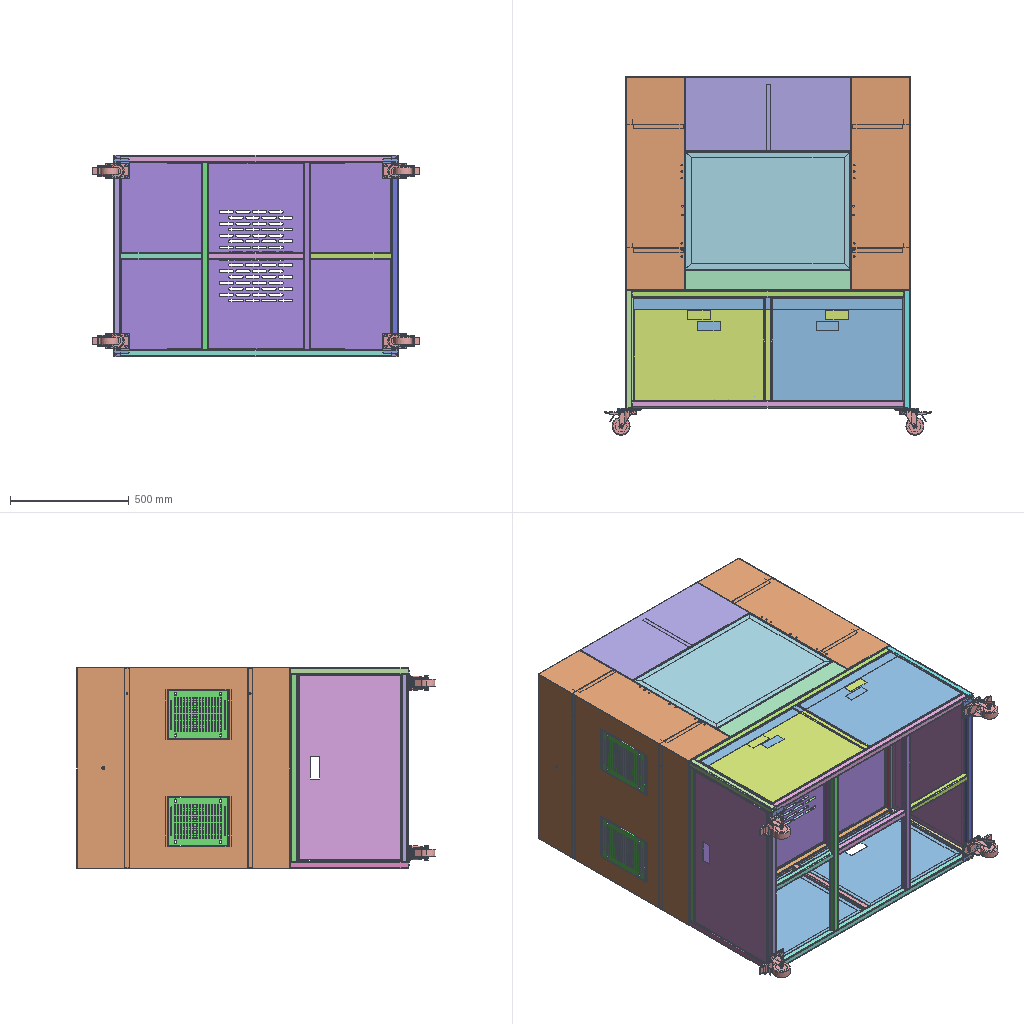Assembly | SolidWorks | 33 different items | 82 placed | box 1381 x 1511 x 850 mm
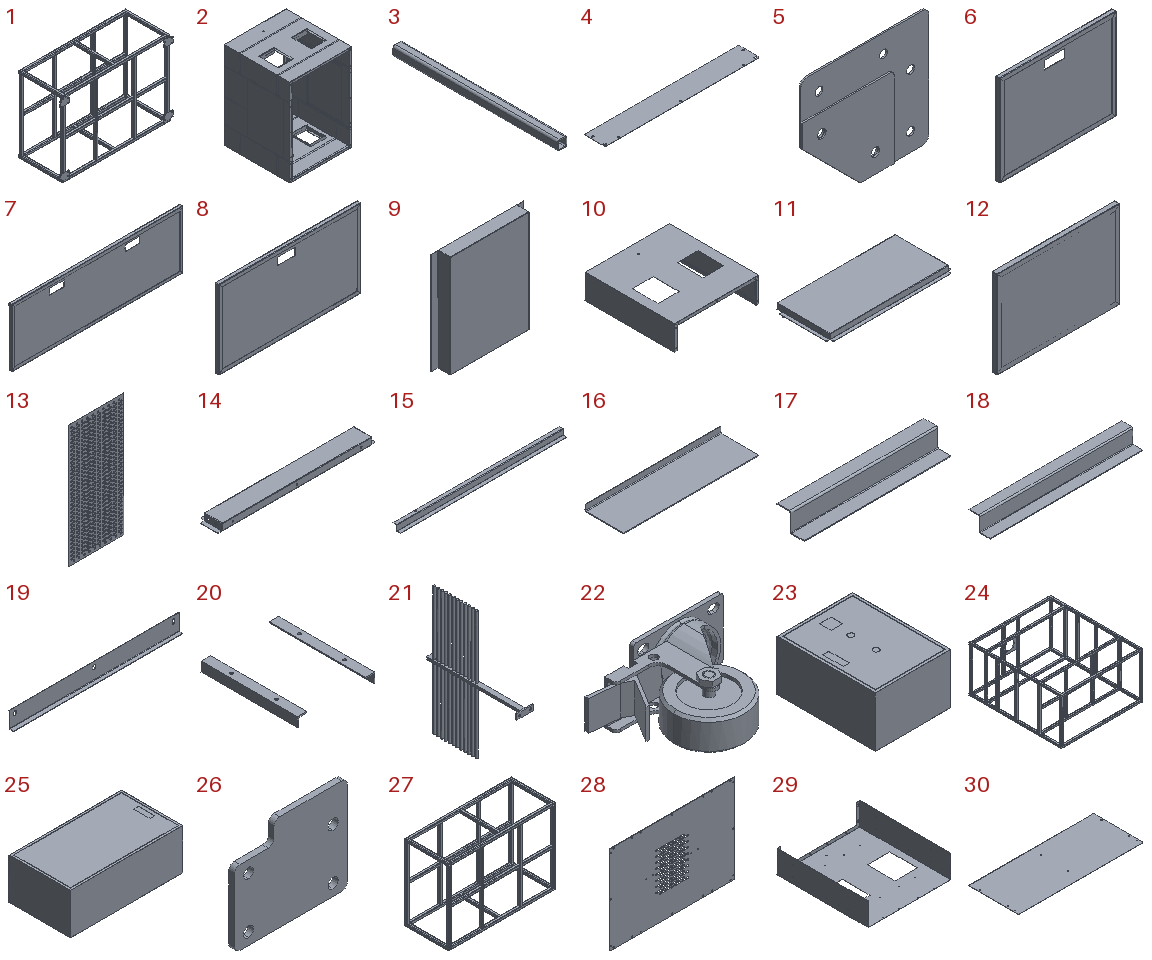Parts list (item | name | quantity | parent item | size | volume | features):
1 | (subassembly) | x1 | - | 1270 x 501 x 850 mm | 4402575 mm3 | features ReferencePattern 2, AEMSimFeature 1, LocalLPattern 1
2 | (subassembly) | x1 | - | 850 x 900 x 1200 mm | 10155913 mm3 | features ReferencePattern 29, MirrorCompFeat 4, LocalLPattern 2, AEMSimFeature 1
3 | - | x1 | - | 30 x 520 x 30 mm | 164668 mm3 | features HoleWzd 1, ICE 1, WeldMemberFeat 1, WeldmentFeature 1
4 | - | x2 | in 2 | 745 x 100 x 1.2 mm | 88883 mm3 | features EdgeFlange 2, Fillet 1, FlatPattern 1, HoleWzd 1, ICE 1, SMBaseFlange 1, SheetMetal 1
5 | - | x1 | - | 99 x 2.4 x 90.5 mm | 13339 mm3 | features ICE 9, EdgeFlange 2, Fillet 2, HoleWzd 2, FlatPattern 1, SMBaseFlange 1, SheetMetal 1, WeldmentFeature 1
6 | - | x4 | - | 552 x 20 x 432 mm | 364714 mm3 | features EdgeFlange 2, FlatPattern 1, ICE 1, SMBaseFlange 1, SheetMetal 1
7 | - | x1 | - | 1135 x 20 x 386 mm | 646370 mm3 | features EdgeFlange 2, FlatPattern 1, ICE 1, SMBaseFlange 1, SheetMetal 1
8 | - | x2 | - | 782 x 20 x 432 mm | 503943 mm3 | features EdgeFlange 2, FlatPattern 1, ICE 1, SMBaseFlange 1, SheetMetal 1
9 | - | x1 | in 1 | 457 x 62.2 x 504.4 mm | 401697 mm3 | features EdgeFlange 2, FlatPattern 1, SMBaseFlange 1, SheetMetal 1
10 | - | x2 | in 2 | 850 x 900 x 250 mm | 1614034 mm3 | features EdgeFlange 8, ICE 5, HoleWzd 4, Fillet 1, FlatPattern 1, LPattern 1, SMBaseFlange 1, SheetMetal 1
11 | - | x2 | in 2 | 737.6 x 333.8 x 60.8 mm | 412436 mm3 | features EdgeFlange 5, ICE 2, Fillet 1, FlatPattern 1, HoleWzd 1, SMBaseFlange 1, SheetMetal 1
12 | - | x2 | in 2 | 696 x 29.2 x 496 mm | 963992 mm3 | features EdgeFlange 2, FlatPattern 1, HoleWzd 1, ICE 1, SMBaseFlange 1, SheetMetal 1
13 | - | x1 | - | 497 x 1.2 x 1097 mm | 505811 mm3 | features LPattern 2, FlatPattern 1, ICE 1, SMBaseFlange 1, SheetMetal 1
14 | - | x2 | in 2 | 737.6 x 103.8 x 32 mm | 156480 mm3 | features EdgeFlange 6, Fillet 1, FlatPattern 1, HoleWzd 1, ICE 1, SMBaseFlange 1, SheetMetal 1
15 | - | x4 | in 2 | 843 x 38.8 x 28.5 mm | 65431 mm3 | features EdgeFlange 2, FlatPattern 1, HoleWzd 1, SMBaseFlange 1, SheetMetal 1
16 | - | x8 | in 2 | 209 x 60 x 10 mm | 17083 mm3 | features EdgeFlange 1, FlatPattern 1, HoleWzd 1, SMBaseFlange 1, SheetMetal 1
17 | - | x8 | in 2 | 210 x 38.8 x 28 mm | 16185 mm3 | features EdgeFlange 2, FlatPattern 1, HoleWzd 1, SMBaseFlange 1, SheetMetal 1
18 | - | x2 | in 2 | 281 x 38.8 x 28 mm | 21657 mm3 | features EdgeFlange 2, FlatPattern 1, HoleWzd 1, SMBaseFlange 1, SheetMetal 1
19 | - | x4 | in 2 | 460 x 12 x 45 mm | 30158 mm3 | features EdgeFlange 2, Fillet 1, FlatPattern 1, ICE 1, LPattern 1, SMBaseFlange 1, SheetMetal 1
20 | - | x1 | in 2 | 205 x 255 x 25 mm | 72570 mm3 | features HoleWzd 1, WeldMemberFeat 1, WeldmentFeature 1
21 | - | x2 | - | 90 x 526 x 700 mm | 1128275 mm3 | features ICE 4, Extrusion 1, HoleWzd 1, LPattern 1
22 | - | x4 | in 1 | 152.5 x 108 x 64 mm | 200603 mm3 | features BaseBody 1
23 | - | x1 | - | 300 x 390 x 201 mm | 697946 mm3 | features ICE 2, Extrusion 1, Shell 1
24 | - | x1 | in 1 | 1200 x 1370 x 680 mm | 7177358 mm3 | features 3DProfileFeature 1, HoleWzd 1, ICE 1, WeldMemberFeat 1, WeldmentFeature 1
25 | - | x1 | - | 550 x 300 x 201 mm | 911866 mm3 | features ICE 3, Extrusion 1, Shell 1
26 | - | x4 | in 1 | 100 x 5 x 85 mm | 37795 mm3 | features Fillet 2, Extrusion 1, HoleWzd 1, ICE 1
27 | - | x1 | in 1 | 1200 x 495 x 850 mm | 4251393 mm3 | features WeldCornerFeat 2, 3DProfileFeature 1, WeldMemberFeat 1, WeldmentFeature 1
28 | - | x1 | - | 1196 x 1.2 x 846 mm | 1157126 mm3 | features LPattern 4, HoleWzd 3, EdgeFlange 1, Fillet 1, FlatPattern 1, ICE 1, SMBaseFlange 1, SheetMetal 1
29 | - | x2 | in 2 | 787 x 866 x 220 mm | 1173690 mm3 | features ICE 6, HoleWzd 5, EdgeFlange 4, LPattern 2, Fillet 1, FlatPattern 1, SMBaseFlange 1, SheetMetal 1
30 | - | x2 | in 2 | 745 x 300 x 30 mm | 291345 mm3 | features EdgeFlange 2, HoleWzd 2, Fillet 1, FlatPattern 1, SMBaseFlange 1, SheetMetal 1
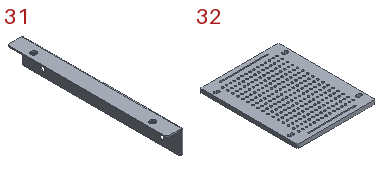31 | - | x8 | in 2 | 26 x 255 x 40 mm | 31191 mm3 | features ICE 2, EdgeFlange 1, Fillet 1, FlatPattern 1, SMBaseFlange 1, SheetMetal 1
32 | - | x4 | - | 200 x 250 x 10 mm | 441110 mm3 | features ICE 3, LPattern 3, Chamfer 1, Extrusion 1
33 | CBAhxj04-2 | x1 | - | - | - | -
Mates (type | each side: item.copy, entity, surface, feature):
In the top assembly
Coincident | 24.1 face plane Square Tube 30 X 30 X 2.6(1) | assembly face | 12 times
Coincident | 24.1 face plane Boss-Extrude1 | assembly face
Concentric | 24.1 face cylinder Boss-Extrude1 | assembly face
Concentric | 24.1 face cylinder M10 Tapped Hole1 | assembly face
DistanceDim | 27.1 face plane Square Tube 30 X 30 X 2.6 - missing(1) | 10.1 face plane Edge-Flange2
Coincident | 27.1 face plane Square Tube 30 X 30 X 2.6 - missing(1) | 10.1 face plane Base-Flange1
Coincident | 27.1 face plane Square Tube 30 X 30 X 2.6 - missing(1) | 10.1 face plane Edge-Flange1
Coincident | 27.1 face plane Square Tube 30 X 30 X 2.6 - missing(1) | 21.1 face plane Boss-Extrude3
Coincident | 27.1 face plane Square Tube 30 X 30 X 2.6 - missing(1) | 21.1 face plane Boss-Extrude1
Coincident | 21.1 face plane Boss-Extrude3 | 21.2 face plane Boss-Extrude3
Coincident | 27.1 face plane Square Tube 30 X 30 X 2.6 - missing(1) | 21.2 face plane Boss-Extrude1
Coincident | 21.1 face plane Boss-Extrude1 | 21.2 face plane Boss-Extrude1
DistanceDim | 27.1 face plane Square Tube 30 X 30 X 2.6 - missing(1) | 28.1 face plane Base-Flange1 | 2 times
Coincident | 28.1 face plane Base-Flange1 | assembly face
Coincident | 29.1 face plane Base-Flange1 | assembly face
Coincident | 28.1 face plane Base-Flange1 | 31.1 face
Coincident | 29.1 face plane Base-Flange1 | 31.1 face
Coincident | 29.2 face plane Base-Flange1 | 31.2 face
Coincident | 28.1 face plane Base-Flange1 | 31.2 face
Coincident | 31.1 face | 31.2 face
Width | 27.1 face plane Square Tube 30 X 30 X 2.6 - missing(1) | 27.1 face plane Square Tube 30 X 30 X 2.6 - missing(1) | 21.2 face plane Boss-Extrude1 | 21.2 face plane Boss-Extrude1
Coincident | 10.2 face plane Edge-Flange1 | 23.1 face
Coincident | 27.1 face plane Square Tube 30 X 30 X 2.6 - missing(1) | 23.1 face | 2 times
Coincident | 27.1 face plane Square Tube 30 X 30 X 2.6 - missing(1) | 6.1 face plane Edge-Flange1
DistanceDim | 6.1 face plane Edge-Flange1 | 27.1 face plane Square Tube 30 X 30 X 2.6 - missing(1)
Coincident | 27.1 face plane Square Tube 30 X 30 X 2.6 - missing(1) | 6.1 face plane Base-Flange1
Coincident | 27.1 face plane Square Tube 30 X 30 X 2.6 - missing(1) | 7.1 face plane Base-Flange1
Coincident | 27.1 face plane Square Tube 30 X 30 X 2.6 - missing(1) | 7.1 face plane Edge-Flange1
DistanceDim | 7.1 face plane Edge-Flange1 | 27.1 face plane Square Tube 30 X 30 X 2.6 - missing(1)
Coincident | 27.1 face plane Square Tube 30 X 30 X 2.6 - missing(1) | 8.1 face plane Edge-Flange1
Coincident | 27.1 face plane Square Tube 30 X 30 X 2.6 - missing(1) | 8.1 face plane Base-Flange1
DistanceDim | 8.1 face plane Edge-Flange1 | 27.1 face plane Square Tube 30 X 30 X 2.6 - missing(1)
Coincident | 27.1 face plane Square Tube 30 X 30 X 2.6 - missing(1) | 8.2 face plane Base-Flange1
Coincident | 27.1 face plane Square Tube 30 X 30 X 2.6 - missing(1) | 8.2 face plane Edge-Flange1
DistanceDim | 8.2 face plane Edge-Flange1 | 27.1 face plane Square Tube 30 X 30 X 2.6 - missing(1)
Coincident | 27.1 face plane Square Tube 30 X 30 X 2.6 - missing(1) | 28.1 face plane Base-Flange1
Coincident | 10.2 face plane Edge-Flange1 | 25.1 face
Coincident | 10.2 face plane Base-Flange1 | 25.1 face
Coincident | 10.2 face plane Edge-Flange2 | 5.1 face
Coincident | 10.2 face plane Edge-Flange2 | 5.2 face
DistanceDim | 10.1 face plane Edge-Flange2 | 5.3 face
Width | 3.1 face plane Square Tube 30 X 30 X 3.2(1) | 3.1 face plane Square Tube 30 X 30 X 3.2(1) | 21.2 face plane Boss-Extrude1 | 21.2 face plane Boss-Extrude1 | 2 times
Coincident | 21.2 face plane Boss-Extrude3 | 3.1 face plane Square Tube 30 X 30 X 3.2(1)
Coincident | 6.1 face plane Base-Flange1 | 6.2 face plane Base-Flange1
DistanceDim | 6.2 face plane Edge-Flange1 | 27.1 face plane Square Tube 30 X 30 X 2.6 - missing(1)
Coincident | 6.1 face plane Edge-Flange1 | 6.2 face plane Edge-Flange1
Coincident | 27.1 face plane Square Tube 30 X 30 X 2.6 - missing(1) | 6.3 face plane Base-Flange1
DistanceDim | 6.3 face plane Edge-Flange1 | 27.1 face plane Square Tube 30 X 30 X 2.6 - missing(1)
Coincident | 27.1 face plane Square Tube 30 X 30 X 2.6 - missing(1) | 6.3 face plane Edge-Flange1
Coincident | 6.3 face plane Base-Flange1 | 6.4 face plane Base-Flange1
DistanceDim | 6.4 face plane Edge-Flange1 | 27.1 face plane Square Tube 30 X 30 X 2.6 - missing(1)
Coincident | 6.3 face plane Edge-Flange1 | 6.4 face plane Edge-Flange1
Coincident | 31.3 face plane Base-Flange1 | 32.1 face plane Boss-Extrude1
Slot | 32.1 face cylinder Cut-Extrude3 | 31.3 face cylinder Cut-Extrude2 | 2 times
Parallel | 10.1 face plane Edge-Flange1 | 32.2 face plane Boss-Extrude1
Coincident | 31.4 face plane Base-Flange1 | 32.3 face plane Boss-Extrude1
Slot | 32.3 face cylinder Cut-Extrude3 | 31.4 face cylinder Cut-Extrude2
Slot | 32.3 face cylinder Cut-Extrude3 | 31.5 face cylinder Cut-Extrude2
In subassembly 2
Coincident | 10.3 face plane Edge-Flange1 | 10.4 face plane Edge-Flange1
DistanceDim | 10.3 face plane Base-Flange1 | 10.4 face plane Base-Flange1
Coincident | 10.3 face plane Edge-Flange2 | 10.4 face plane Edge-Flange2
Coincident | 10.3 face plane Edge-Flange1 | 11.1 face plane Base-Flange1
Coincident | 10.3 face plane Edge-Flange2 | 11.1 face plane Edge-Flange1 | 2 times
Coincident | 10.4 face plane Edge-Flange1 | 11.2 face plane Base-Flange1
Coincident | 10.4 face plane Edge-Flange2 | 11.2 face plane Edge-Flange1
Coincident | 10.3 face plane Edge-Flange9 | 29.3 face plane Base-Flange1
DistanceDim | 29.3 face plane Edge-Flange1 | 10.3 face plane Edge-Flange8
Coincident | 10.4 face plane Edge-Flange9 | 29.4 face plane Base-Flange1
Coincident | 29.3 face plane Edge-Flange1 | 29.4 face plane Edge-Flange1
Coincident | 11.2 face plane Edge-Flange5 | 30.1 face plane Base-Flange1
Coincident | 11.2 face plane Base-Flange1 | 12.1 face plane Base-Flange1
DistanceDim | 12.1 face plane Edge-Flange1 | 14.1 face plane Edge-Flange1
DistanceDim | 12.1 face plane Edge-Flange1 | 10.3 face plane Edge-Flange2
DistanceDim | 12.2 face plane Edge-Flange1 | 10.3 face plane Edge-Flange2
Coincident | 11.1 face plane Base-Flange1 | 12.2 face plane Boss-Extrude1
Coincident | 10.3 face plane Base-Flange1 | 15.1 face plane Edge-Flange2
DistanceDim | 10.3 face plane Edge-Flange2 | 15.1 face plane Edge-Flange1
DistanceDim | 15.1 face plane Edge-Flange1 | 10.3 face plane Edge-Flange1
Coincident | 10.3 face plane Edge-Flange2 | 29.3 face plane Edge-Flange1
Coincident | 10.4 face plane Edge-Flange2 | 29.4 face plane Edge-Flange1
DistanceDim | 10.3 face plane Cut-Extrude1 | 16.1 face plane Base-Flange1
Coincident | 10.3 face plane Base-Flange1 | 16.1 face plane Edge-Flange1
Coincident | 10.3 face plane Base-Flange1 | 16.2 face plane Edge-Flange1
DistanceDim | 10.3 face plane Cut-Extrude1 | 16.2 face plane Base-Flange1
Coincident | 11.1 face plane Edge-Flange1 | 11.2 face plane Edge-Flange1
Coincident | 10.4 face plane Edge-Flange1 | 14.1 face plane Base-Flange1
Coincident | 10.3 face plane Edge-Flange2 | 14.1 face plane Edge-Flange1
Coincident | 10.4 face plane Edge-Flange2 | 14.1 face plane Edge-Flange1
Coincident | 14.1 face plane Edge-Flange1 | 14.2 face plane Edge-Flange1
Coincident | 10.3 face plane Edge-Flange1 | 14.2 face plane Base-Flange1
Coincident | 10.4 face plane Edge-Flange2 | 14.2 face plane Edge-Flange1
Coincident | 29.3 face plane Edge-Flange2 | 30.1 face plane Edge-Flange1
DistanceDim | 10.3 face plane Edge-Flange2 | 30.1 face plane Edge-Flange1
Coincident | 14.2 face plane Edge-Flange2 | 4.1 face plane Base-Flange1
Coincident | 14.1 face plane Edge-Flange2 | 4.2 face plane Base-Flange1
DistanceDim | 29.3 face plane Edge-Flange1 | 4.2 face plane Base-Flange1
DistanceDim | 29.4 face plane Edge-Flange1 | 4.2 face plane Base-Flange1
Coincident | 4.1 face plane Base-Flange1 | 4.2 face plane Base-Flange1
DistanceDim | 14.2 face plane Edge-Flange1 | 12.2 face plane Edge-Flange1
Coincident | 10.3 face plane Edge-Flange1 | 17.1 face plane Edge-Flange2
Coincident | 15.1 face plane Edge-Flange1 | 17.1 face plane Edge-Flange1
DistanceDim | 17.1 face plane Base-Flange1 | 15.1 face plane Base-Flange1
Coincident | 10.3 face plane Edge-Flange1 | 17.2 face plane Edge-Flange2
Coincident | 15.1 face plane Edge-Flange1 | 17.2 face plane Edge-Flange1
Coincident | 15.1 face plane Base-Flange1 | 17.2 face plane Base-Flange1
Coincident | 11.1 face plane Base-Flange1 | 18.1 face plane Edge-Flange2
Coincident | 11.1 face plane Edge-Flange3 | 18.1 face plane Edge-Flange1
Coincident | 11.2 face plane Base-Flange1 | 18.2 face plane Edge-Flange2
Coincident | 11.2 edge | 18.2 face plane Edge-Flange1
Coincident | 14.1 face plane Edge-Flange2 | 19.1 face plane Edge-Flange1
DistanceDim | 10.4 face plane Edge-Flange2 | 19.1 face plane Base-Flange1
Coincident | 19.1 face plane Edge-Flange1 | 19.2 face plane Edge-Flange1
DistanceDim | 19.2 face plane Base-Flange1 | 10.3 face plane Edge-Flange2
DistanceDim | 20.1 face | 10.4 face plane Base-Flange1
Coincident | 16.3 face plane Base-Flange1 | 20.1 face
DistanceDim | 19.1 face plane Edge-Flange1 | 14.1 face plane Edge-Flange2
Coincident | 19.1 face plane Base-Flange1 | 19.2 face plane Base-Flange1
DistanceDim | 31.6 face plane Base-Flange1 | 10.4 face plane Base-Flange1
Coincident | 31.6 face plane Base-Flange1 | 31.1 face plane Base-Flange1
Coincident | 31.6 face plane Edge Bend1 | 31.1 face plane Edge-Flange1
Slot | 30.2 face cylinder M4 Clearance Hole1 | 11.1 face cylinder Cut-Extrude2
Parallel | 11.1 face plane Edge-Flange3 | 30.2 face plane Base-Flange1
Coincident | 29.4 face plane Edge-Flange2 | 30.2 face plane Edge-Flange1
Coincident | 16.1 face plane Base-Flange1 | 16.2 face plane Base-Flange1
In subassembly 1
Coincident | 24.2 face plane Square Tube 30 X 30 X 2.6(1) | 26.1 face plane Boss-Extrude1
DistanceDim | 26.1 face plane Boss-Extrude1 | 24.2 face plane Square Tube 30 X 30 X 2.6(1) | 2 times
Coincident | 22.1 face plane Input1 | 26.1 face plane Boss-Extrude1
DistanceDim | 22.1 face plane Input1 | 26.1 face plane Boss-Extrude1 | 2 times
Coincident | 26.1 face plane Boss-Extrude1 | 26.2 face plane Boss-Extrude1 | 2 times
DistanceDim | 26.3 face plane Boss-Extrude1 | 24.2 face plane Square Tube 30 X 30 X 2.6(1)
Coincident | 24.2 face plane Square Tube 30 X 30 X 2.6(1) | 26.3 face plane Cut-Extrude1
Coincident | 24.2 face plane Square Tube 30 X 30 X 2.6(1) | 26.4 face plane Cut-Extrude1
Coincident | 26.3 face plane Boss-Extrude1 | 26.4 face plane Boss-Extrude1
Coincident | 26.1 face plane Boss-Extrude1 | 26.3 face plane Boss-Extrude1
Coincident | 26.3 face plane Boss-Extrude1 | 22.2 face plane Input1
DistanceDim | 22.2 face plane Input1 | 26.3 face plane Cut-Extrude1
DistanceDim | 26.3 face plane Boss-Extrude1 | 22.2 edge
Coincident | 24.2 face plane Square Tube 30 X 30 X 2.6(1) | 27.2 face plane Square Tube 30 X 30 X 2.6 - missing(1) | 3 times
Coincident | 27.2 face plane Square Tube 30 X 30 X 2.6 - missing(1) | 9.1 face plane Edge-Flange2
Width | 9.1 face plane Edge-Flange1 | 9.1 face plane Edge-Flange1 | 27.2 face plane Square Tube 30 X 30 X 2.6 - missing(1) | 27.2 face plane Square Tube 30 X 30 X 2.6 - missing(1) | 2 times
Slot | 26.2 face cylinder M8 Clearance Hole1 | 22.3 face cylinder Input1
Slot | 26.4 face cylinder M8 Clearance Hole1 | 22.4 face cylinder Input1